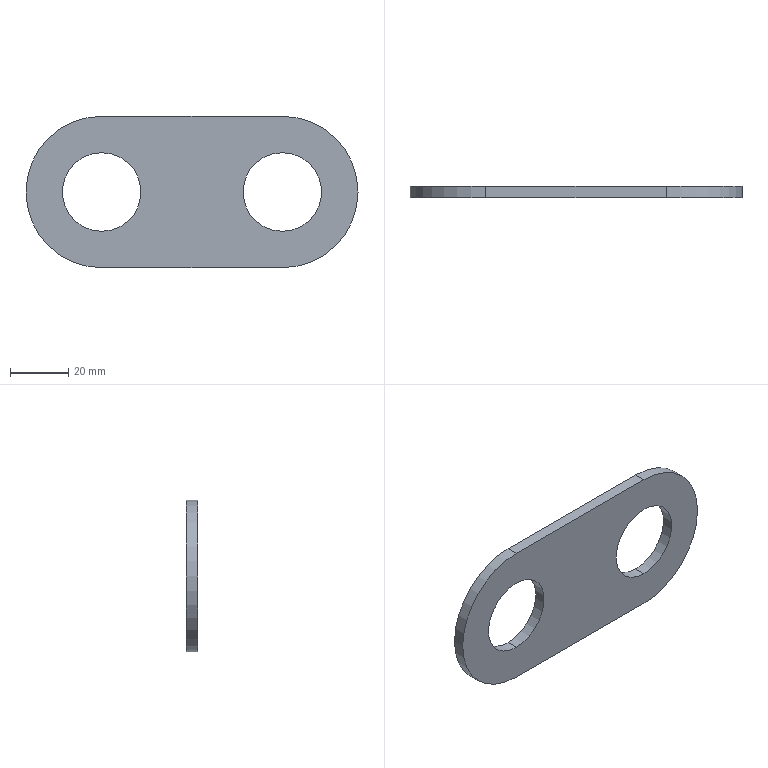Part | SolidWorks | features Extrusion 1 | 1 solid | 10 faces | box 114 x 4 x 52 mm | volume 16810 mm3 | cylinder 6 | plane 4 | commonest cylinder face diameters 27 x4 52 x2
STEP:
#1=CARTESIAN_POINT('',(-62.,2.,-13.5));
#2=VERTEX_POINT('',#1);
#3=CARTESIAN_POINT('',(-62.,2.,13.5));
#4=VERTEX_POINT('',#3);
#5=CARTESIAN_POINT('',(-62.,2.,0.));
#6=DIRECTION('',(0.,1.,0.));
#7=DIRECTION('',(0.,0.,1.));
#8=AXIS2_PLACEMENT_3D('',#5,#6,#7);
#9=CIRCLE('',#8,13.5);
#10=EDGE_CURVE('',#2,#4,#9,.T.);
#11=ORIENTED_EDGE('',*,*,#10,.T.);
#12=CARTESIAN_POINT('',(-62.,-2.,13.5));
#13=VERTEX_POINT('',#12);
#14=CARTESIAN_POINT('',(-62.,2.,13.5));
#15=DIRECTION('',(0.,-1.,0.));
#16=VECTOR('',#15,1000.);
#17=LINE('',#14,#16);
#18=EDGE_CURVE('',#4,#13,#17,.T.);
#19=ORIENTED_EDGE('',*,*,#18,.T.);
#20=CARTESIAN_POINT('',(-62.,-2.,-13.5));
#21=VERTEX_POINT('',#20);
#22=CARTESIAN_POINT('',(-62.,-2.,0.));
#23=DIRECTION('',(0.,1.,0.));
#24=DIRECTION('',(0.,0.,1.));
#25=AXIS2_PLACEMENT_3D('',#22,#23,#24);
#26=CIRCLE('',#25,13.5);
#27=EDGE_CURVE('',#21,#13,#26,.T.);
#28=ORIENTED_EDGE('',*,*,#27,.F.);
#29=CARTESIAN_POINT('',(-62.,2.,-13.5));
#30=DIRECTION('',(0.,-1.,0.));
#31=VECTOR('',#30,1000.);
#32=LINE('',#29,#31);
#33=EDGE_CURVE('',#2,#21,#32,.T.);
#34=ORIENTED_EDGE('',*,*,#33,.F.);
#35=EDGE_LOOP('',(#11,#19,#28,#34));
#36=FACE_OUTER_BOUND('',#35,.T.);
#37=CARTESIAN_POINT('',(-62.,2.,0.));
#38=DIRECTION('',(0.,-1.,0.));
#39=DIRECTION('',(0.,0.,-1.));
#40=AXIS2_PLACEMENT_3D('',#37,#38,#39);
#41=CYLINDRICAL_SURFACE('',#40,13.5);
#42=ADVANCED_FACE('',(#36),#41,.F.);
#43=CARTESIAN_POINT('',(0.,2.,-13.5));
#44=VERTEX_POINT('',#43);
#45=CARTESIAN_POINT('',(0.,2.,13.5));
#46=VERTEX_POINT('',#45);
#47=CARTESIAN_POINT('',(0.,2.,0.));
#48=DIRECTION('',(0.,1.,0.));
#49=DIRECTION('',(0.,0.,1.));
#50=AXIS2_PLACEMENT_3D('',#47,#48,#49);
#51=CIRCLE('',#50,13.5);
#52=EDGE_CURVE('',#44,#46,#51,.T.);
#53=ORIENTED_EDGE('',*,*,#52,.T.);
#54=CARTESIAN_POINT('',(0.,-2.,13.5));
#55=VERTEX_POINT('',#54);
#56=CARTESIAN_POINT('',(0.,2.,13.5));
#57=DIRECTION('',(0.,-1.,0.));
#58=VECTOR('',#57,1000.);
#59=LINE('',#56,#58);
#60=EDGE_CURVE('',#46,#55,#59,.T.);
#61=ORIENTED_EDGE('',*,*,#60,.T.);
#62=CARTESIAN_POINT('',(0.,-2.,-13.5));
#63=VERTEX_POINT('',#62);
#64=CARTESIAN_POINT('',(0.,-2.,0.));
#65=DIRECTION('',(0.,1.,0.));
#66=DIRECTION('',(0.,0.,1.));
#67=AXIS2_PLACEMENT_3D('',#64,#65,#66);
#68=CIRCLE('',#67,13.5);
#69=EDGE_CURVE('',#63,#55,#68,.T.);
#70=ORIENTED_EDGE('',*,*,#69,.F.);
#71=CARTESIAN_POINT('',(0.,2.,-13.5));
#72=DIRECTION('',(0.,-1.,0.));
#73=VECTOR('',#72,1000.);
#74=LINE('',#71,#73);
#75=EDGE_CURVE('',#44,#63,#74,.T.);
#76=ORIENTED_EDGE('',*,*,#75,.F.);
#77=EDGE_LOOP('',(#53,#61,#70,#76));
#78=FACE_OUTER_BOUND('',#77,.T.);
#79=CARTESIAN_POINT('',(0.,2.,0.));
#80=DIRECTION('',(0.,-1.,0.));
#81=DIRECTION('',(0.,0.,-1.));
#82=AXIS2_PLACEMENT_3D('',#79,#80,#81);
#83=CYLINDRICAL_SURFACE('',#82,13.5);
#84=ADVANCED_FACE('',(#78),#83,.F.);
#85=ORIENTED_EDGE('',*,*,#52,.F.);
#86=CARTESIAN_POINT('',(0.,2.,0.));
#87=DIRECTION('',(0.,1.,0.));
#88=DIRECTION('',(0.,0.,1.));
#89=AXIS2_PLACEMENT_3D('',#86,#87,#88);
#90=CIRCLE('',#89,13.5);
#91=EDGE_CURVE('',#46,#44,#90,.T.);
#92=ORIENTED_EDGE('',*,*,#91,.F.);
#93=EDGE_LOOP('',(#85,#92));
#94=FACE_BOUND('',#93,.T.);
#95=CARTESIAN_POINT('',(-62.,2.,-26.));
#96=VERTEX_POINT('',#95);
#97=CARTESIAN_POINT('',(-62.,2.,26.));
#98=VERTEX_POINT('',#97);
#99=CARTESIAN_POINT('',(-62.,2.,0.));
#100=DIRECTION('',(0.,1.,0.));
#101=DIRECTION('',(0.,0.,1.));
#102=AXIS2_PLACEMENT_3D('',#99,#100,#101);
#103=CIRCLE('',#102,26.);
#104=EDGE_CURVE('',#96,#98,#103,.T.);
#105=ORIENTED_EDGE('',*,*,#104,.T.);
#106=CARTESIAN_POINT('',(0.,2.,26.));
#107=VERTEX_POINT('',#106);
#108=CARTESIAN_POINT('',(0.,2.,26.));
#109=DIRECTION('',(1.,0.,0.));
#110=VECTOR('',#109,1000.);
#111=LINE('',#108,#110);
#112=EDGE_CURVE('',#98,#107,#111,.T.);
#113=ORIENTED_EDGE('',*,*,#112,.T.);
#114=CARTESIAN_POINT('',(0.,2.,-26.));
#115=VERTEX_POINT('',#114);
#116=CARTESIAN_POINT('',(0.,2.,0.));
#117=DIRECTION('',(0.,1.,0.));
#118=DIRECTION('',(0.,0.,1.));
#119=AXIS2_PLACEMENT_3D('',#116,#117,#118);
#120=CIRCLE('',#119,26.);
#121=EDGE_CURVE('',#107,#115,#120,.T.);
#122=ORIENTED_EDGE('',*,*,#121,.T.);
#123=CARTESIAN_POINT('',(-62.,2.,-26.));
#124=DIRECTION('',(-1.,0.,0.));
#125=VECTOR('',#124,1000.);
#126=LINE('',#123,#125);
#127=EDGE_CURVE('',#115,#96,#126,.T.);
#128=ORIENTED_EDGE('',*,*,#127,.T.);
#129=EDGE_LOOP('',(#105,#113,#122,#128));
#130=FACE_OUTER_BOUND('',#129,.T.);
#131=ORIENTED_EDGE('',*,*,#10,.F.);
#132=CARTESIAN_POINT('',(-62.,2.,0.));
#133=DIRECTION('',(0.,1.,0.));
#134=DIRECTION('',(0.,0.,1.));
#135=AXIS2_PLACEMENT_3D('',#132,#133,#134);
#136=CIRCLE('',#135,13.5);
#137=EDGE_CURVE('',#4,#2,#136,.T.);
#138=ORIENTED_EDGE('',*,*,#137,.F.);
#139=EDGE_LOOP('',(#131,#138));
#140=FACE_BOUND('',#139,.T.);
#141=CARTESIAN_POINT('',(-62.,2.,0.));
#142=DIRECTION('',(0.,1.,0.));
#143=DIRECTION('',(0.,0.,1.));
#144=AXIS2_PLACEMENT_3D('',#141,#142,#143);
#145=PLANE('',#144);
#146=ADVANCED_FACE('',(#94,#130,#140),#145,.T.);
#147=ORIENTED_EDGE('',*,*,#69,.T.);
#148=CARTESIAN_POINT('',(0.,-2.,0.));
#149=DIRECTION('',(0.,1.,0.));
#150=DIRECTION('',(0.,0.,1.));
#151=AXIS2_PLACEMENT_3D('',#148,#149,#150);
#152=CIRCLE('',#151,13.5);
#153=EDGE_CURVE('',#55,#63,#152,.T.);
#154=ORIENTED_EDGE('',*,*,#153,.T.);
#155=EDGE_LOOP('',(#147,#154));
#156=FACE_BOUND('',#155,.T.);
#157=CARTESIAN_POINT('',(-62.,-2.,-26.));
#158=VERTEX_POINT('',#157);
#159=CARTESIAN_POINT('',(-62.,-2.,26.));
#160=VERTEX_POINT('',#159);
#161=CARTESIAN_POINT('',(-62.,-2.,0.));
#162=DIRECTION('',(0.,1.,0.));
#163=DIRECTION('',(0.,0.,1.));
#164=AXIS2_PLACEMENT_3D('',#161,#162,#163);
#165=CIRCLE('',#164,26.);
#166=EDGE_CURVE('',#158,#160,#165,.T.);
#167=ORIENTED_EDGE('',*,*,#166,.F.);
#168=CARTESIAN_POINT('',(0.,-2.,-26.));
#169=VERTEX_POINT('',#168);
#170=CARTESIAN_POINT('',(-62.,-2.,-26.));
#171=DIRECTION('',(-1.,0.,0.));
#172=VECTOR('',#171,1000.);
#173=LINE('',#170,#172);
#174=EDGE_CURVE('',#169,#158,#173,.T.);
#175=ORIENTED_EDGE('',*,*,#174,.F.);
#176=CARTESIAN_POINT('',(0.,-2.,26.));
#177=VERTEX_POINT('',#176);
#178=CARTESIAN_POINT('',(0.,-2.,0.));
#179=DIRECTION('',(0.,1.,0.));
#180=DIRECTION('',(0.,0.,1.));
#181=AXIS2_PLACEMENT_3D('',#178,#179,#180);
#182=CIRCLE('',#181,26.);
#183=EDGE_CURVE('',#177,#169,#182,.T.);
#184=ORIENTED_EDGE('',*,*,#183,.F.);
#185=CARTESIAN_POINT('',(0.,-2.,26.));
#186=DIRECTION('',(1.,0.,0.));
#187=VECTOR('',#186,1000.);
#188=LINE('',#185,#187);
#189=EDGE_CURVE('',#160,#177,#188,.T.);
#190=ORIENTED_EDGE('',*,*,#189,.F.);
#191=EDGE_LOOP('',(#167,#175,#184,#190));
#192=FACE_OUTER_BOUND('',#191,.T.);
#193=ORIENTED_EDGE('',*,*,#27,.T.);
#194=CARTESIAN_POINT('',(-62.,-2.,0.));
#195=DIRECTION('',(0.,1.,0.));
#196=DIRECTION('',(0.,0.,1.));
#197=AXIS2_PLACEMENT_3D('',#194,#195,#196);
#198=CIRCLE('',#197,13.5);
#199=EDGE_CURVE('',#13,#21,#198,.T.);
#200=ORIENTED_EDGE('',*,*,#199,.T.);
#201=EDGE_LOOP('',(#193,#200));
#202=FACE_BOUND('',#201,.T.);
#203=CARTESIAN_POINT('',(-62.,-2.,0.));
#204=DIRECTION('',(0.,1.,0.));
#205=DIRECTION('',(0.,0.,1.));
#206=AXIS2_PLACEMENT_3D('',#203,#204,#205);
#207=PLANE('',#206);
#208=ADVANCED_FACE('',(#156,#192,#202),#207,.F.);
#209=ORIENTED_EDGE('',*,*,#166,.T.);
#210=CARTESIAN_POINT('',(-62.,2.,26.));
#211=DIRECTION('',(0.,-1.,0.));
#212=VECTOR('',#211,1000.);
#213=LINE('',#210,#212);
#214=EDGE_CURVE('',#98,#160,#213,.T.);
#215=ORIENTED_EDGE('',*,*,#214,.F.);
#216=ORIENTED_EDGE('',*,*,#104,.F.);
#217=CARTESIAN_POINT('',(-62.,2.,-26.));
#218=DIRECTION('',(0.,-1.,0.));
#219=VECTOR('',#218,1000.);
#220=LINE('',#217,#219);
#221=EDGE_CURVE('',#96,#158,#220,.T.);
#222=ORIENTED_EDGE('',*,*,#221,.T.);
#223=EDGE_LOOP('',(#209,#215,#216,#222));
#224=FACE_OUTER_BOUND('',#223,.T.);
#225=CARTESIAN_POINT('',(-62.,2.,0.));
#226=DIRECTION('',(0.,-1.,0.));
#227=DIRECTION('',(0.,0.,-1.));
#228=AXIS2_PLACEMENT_3D('',#225,#226,#227);
#229=CYLINDRICAL_SURFACE('',#228,26.);
#230=ADVANCED_FACE('',(#224),#229,.T.);
#231=ORIENTED_EDGE('',*,*,#189,.T.);
#232=CARTESIAN_POINT('',(0.,2.,26.));
#233=DIRECTION('',(0.,-1.,0.));
#234=VECTOR('',#233,1000.);
#235=LINE('',#232,#234);
#236=EDGE_CURVE('',#107,#177,#235,.T.);
#237=ORIENTED_EDGE('',*,*,#236,.F.);
#238=ORIENTED_EDGE('',*,*,#112,.F.);
#239=ORIENTED_EDGE('',*,*,#214,.T.);
#240=EDGE_LOOP('',(#231,#237,#238,#239));
#241=FACE_OUTER_BOUND('',#240,.T.);
#242=CARTESIAN_POINT('',(0.,2.,26.));
#243=DIRECTION('',(0.,0.,-1.));
#244=DIRECTION('',(-1.,0.,0.));
#245=AXIS2_PLACEMENT_3D('',#242,#243,#244);
#246=PLANE('',#245);
#247=ADVANCED_FACE('',(#241),#246,.F.);
#248=ORIENTED_EDGE('',*,*,#183,.T.);
#249=CARTESIAN_POINT('',(0.,2.,-26.));
#250=DIRECTION('',(0.,-1.,0.));
#251=VECTOR('',#250,1000.);
#252=LINE('',#249,#251);
#253=EDGE_CURVE('',#115,#169,#252,.T.);
#254=ORIENTED_EDGE('',*,*,#253,.F.);
#255=ORIENTED_EDGE('',*,*,#121,.F.);
#256=ORIENTED_EDGE('',*,*,#236,.T.);
#257=EDGE_LOOP('',(#248,#254,#255,#256));
#258=FACE_OUTER_BOUND('',#257,.T.);
#259=CARTESIAN_POINT('',(0.,2.,0.));
#260=DIRECTION('',(0.,-1.,0.));
#261=DIRECTION('',(0.,0.,-1.));
#262=AXIS2_PLACEMENT_3D('',#259,#260,#261);
#263=CYLINDRICAL_SURFACE('',#262,26.);
#264=ADVANCED_FACE('',(#258),#263,.T.);
#265=ORIENTED_EDGE('',*,*,#174,.T.);
#266=ORIENTED_EDGE('',*,*,#221,.F.);
#267=ORIENTED_EDGE('',*,*,#127,.F.);
#268=ORIENTED_EDGE('',*,*,#253,.T.);
#269=EDGE_LOOP('',(#265,#266,#267,#268));
#270=FACE_OUTER_BOUND('',#269,.T.);
#271=CARTESIAN_POINT('',(-62.,2.,-26.));
#272=DIRECTION('',(0.,0.,1.));
#273=DIRECTION('',(1.,0.,0.));
#274=AXIS2_PLACEMENT_3D('',#271,#272,#273);
#275=PLANE('',#274);
#276=ADVANCED_FACE('',(#270),#275,.F.);
#277=ORIENTED_EDGE('',*,*,#60,.F.);
#278=ORIENTED_EDGE('',*,*,#91,.T.);
#279=ORIENTED_EDGE('',*,*,#75,.T.);
#280=ORIENTED_EDGE('',*,*,#153,.F.);
#281=EDGE_LOOP('',(#277,#278,#279,#280));
#282=FACE_OUTER_BOUND('',#281,.T.);
#283=CARTESIAN_POINT('',(0.,2.,0.));
#284=DIRECTION('',(0.,-1.,0.));
#285=DIRECTION('',(0.,0.,-1.));
#286=AXIS2_PLACEMENT_3D('',#283,#284,#285);
#287=CYLINDRICAL_SURFACE('',#286,13.5);
#288=ADVANCED_FACE('',(#282),#287,.F.);
#289=ORIENTED_EDGE('',*,*,#18,.F.);
#290=ORIENTED_EDGE('',*,*,#137,.T.);
#291=ORIENTED_EDGE('',*,*,#33,.T.);
#292=ORIENTED_EDGE('',*,*,#199,.F.);
#293=EDGE_LOOP('',(#289,#290,#291,#292));
#294=FACE_OUTER_BOUND('',#293,.T.);
#295=CARTESIAN_POINT('',(-62.,2.,0.));
#296=DIRECTION('',(0.,-1.,0.));
#297=DIRECTION('',(0.,0.,-1.));
#298=AXIS2_PLACEMENT_3D('',#295,#296,#297);
#299=CYLINDRICAL_SURFACE('',#298,13.5);
#300=ADVANCED_FACE('',(#294),#299,.F.);
#301=CLOSED_SHELL('',(#42,#84,#146,#208,#230,#247,#264,#276,#288,#300));
#302=MANIFOLD_SOLID_BREP('',#301);
#303=CARTESIAN_POINT('',(0.,0.,0.));
#304=DIRECTION('',(0.,0.,1.));
#305=DIRECTION('',(1.,0.,0.));
#306=AXIS2_PLACEMENT_3D('',#303,#304,#305);
#307=(LENGTH_UNIT()NAMED_UNIT(*)SI_UNIT(.MILLI.,.METRE.));
#308=UNCERTAINTY_MEASURE_WITH_UNIT(LENGTH_MEASURE(0.00001),#307,'','');
#309=(NAMED_UNIT(*)PLANE_ANGLE_UNIT()SI_UNIT($,.RADIAN.));
#310=(NAMED_UNIT(*)SI_UNIT($,.STERADIAN.)SOLID_ANGLE_UNIT());
#311=(GEOMETRIC_REPRESENTATION_CONTEXT(3)GLOBAL_UNCERTAINTY_ASSIGNED_CONTEXT((#308))GLOBAL_UNIT_ASSIGNED_CONTEXT((#307,#309,#310))REPRESENTATION_CONTEXT('',''));
#312=ADVANCED_BREP_SHAPE_REPRESENTATION('',(#302,#306),#311);